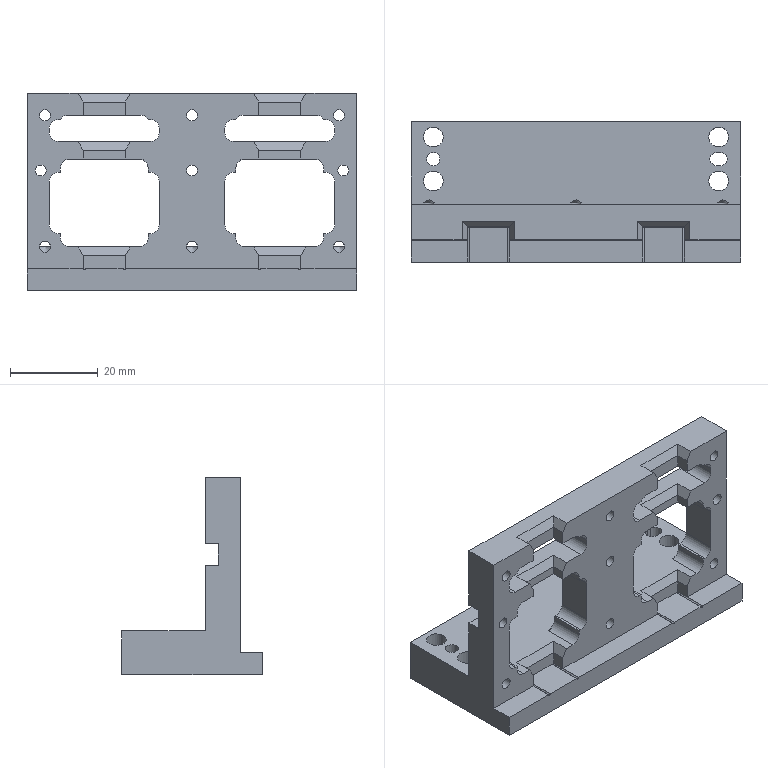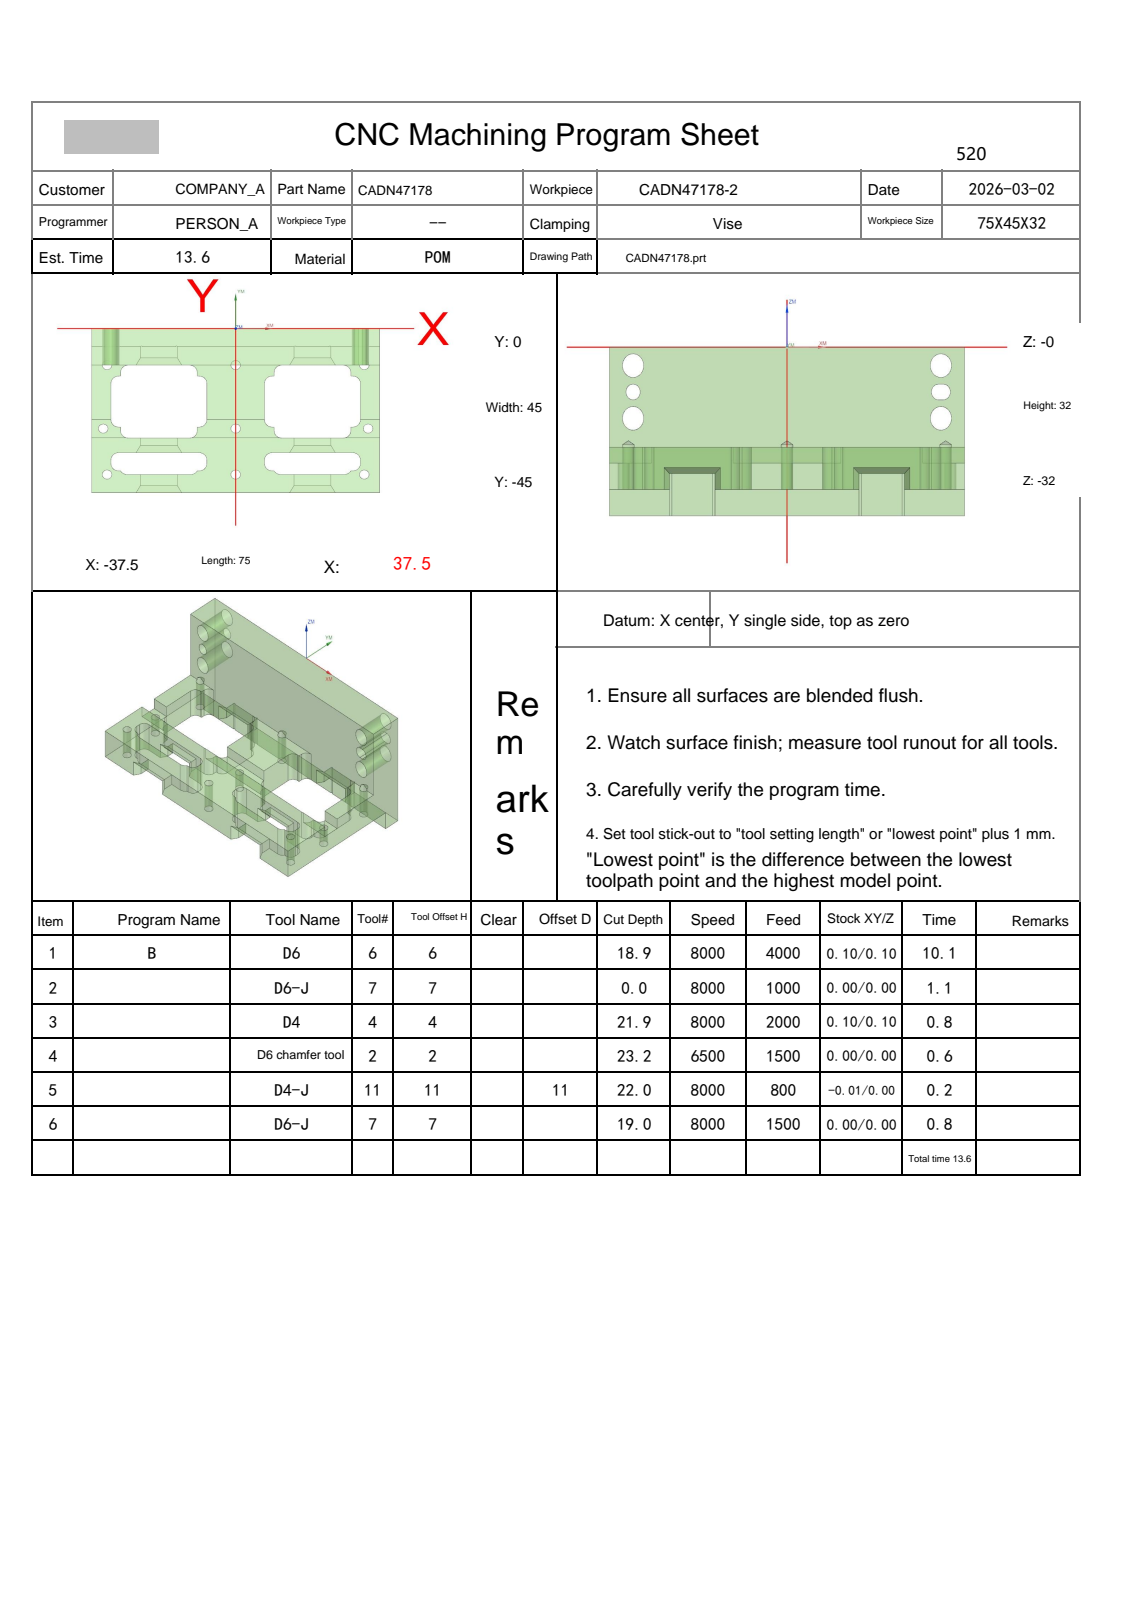NC program | NX | posted by the shop | part box 75 x 32 x 45 mm
Lines 1 to 2828 of 3118, first 1780 of 2826 lines:
%
O0001
(Machine time: 14.54 MIN)
(===Total Tool:5===)
(T6=D6      D=6.   R=0.   D-  H06 Z=-18.9 )
(T7=D6-J    D=6.   R=0.   D-  H07 Z=-19.  )
(T4=D4      D=4.   R=0.   D-  H04 Z=-21.9 )
(T2=D6 chamfer tool   D=6.   R=0.   D-  H02 Z=-23.2 )
(T11=D4-J   D=4.   R=0.   D11 H11 Z=-22.  )
G80 G90 G17 G49 G40
G91 G28 Z0
M01
N1 T06 M06
(D6  D=6. R=0. H=06 ce=0.20 di=0.10)
G00 G90 G54 X52.5 Y-45. M03 S8000
G43 H06 Z50.
M08
Z5.014
G01 Z3.014 F4000.
X40.5
X-39.96
G02 X-40.5 Y-44.46 I0.0 J.54
G01 Y-42.54
G02 X-39.96 Y-42. I.54 J0.0
G01 X39.96
G03 X40.5 Y-41.46 I0.0 J.54
G01 Y-39.54
G03 X39.96 Y-39. I-.54 J0.0
G01 X-39.96
G02 X-40.5 Y-38.46 I0.0 J.54
G01 Y-36.54
G02 X-39.96 Y-36. I.54 J0.0
G01 X39.96
G03 X40.5 Y-35.46 I0.0 J.54
G01 Y-33.54
G03 X39.96 Y-33. I-.54 J0.0
G01 X-39.96
G02 X-40.5 Y-32.46 I0.0 J.54
G01 Y-30.54
G02 X-39.96 Y-30. I.54 J0.0
G01 X39.96
G03 X40.5 Y-29.46 I0.0 J.54
G01 Y-27.54
G03 X39.96 Y-27. I-.54 J0.0
G01 X-39.96
G02 X-40.5 Y-26.46 I0.0 J.54
G01 Y-24.54
G02 X-39.96 Y-24. I.54 J0.0
G01 X39.96
G03 X40.5 Y-23.46 I0.0 J.54
G01 Y-21.54
G03 X39.96 Y-21. I-.54 J0.0
G01 X-39.96
G02 X-40.5 Y-20.46 I0.0 J.54
G01 Y-18.54
G02 X-39.96 Y-18. I.54 J0.0
G01 X39.96
G03 X40.5 Y-17.46 I0.0 J.54
G01 Y-15.54
G03 X39.96 Y-15. I-.54 J0.0
G01 X-39.96
G02 X-40.5 Y-14.46 I0.0 J.54
G01 Y-12.54
G02 X-39.96 Y-12. I.54 J0.0
G01 X39.96
G03 X40.5 Y-11.46 I0.0 J.54
G01 Y-9.54
G03 X39.96 Y-9. I-.54 J0.0
G01 X-39.96
G02 X-40.5 Y-8.46 I0.0 J.54
G01 Y-6.54
G02 X-39.96 Y-6. I.54 J0.0
G01 X39.96
G03 X40.5 Y-5.46 I0.0 J.54
G01 Y-3.54
G03 X39.96 Y-3. I-.54 J0.0
G01 X-39.96
G02 X-40.5 Y-2.46 I0.0 J.54
G01 Y-.54
G02 X-39.96 Y0.0 I.54 J0.0
G01 X40.5
X52.5
Z5.014
G00 Z6.5
Y-45.
Z4.529
G01 Z2.529
X40.5
X-39.96
G02 X-40.5 Y-44.46 I0.0 J.54
G01 Y-42.54
G02 X-39.96 Y-42. I.54 J0.0
G01 X39.96
G03 X40.5 Y-41.46 I0.0 J.54
G01 Y-39.54
G03 X39.96 Y-39. I-.54 J0.0
G01 X-39.96
G02 X-40.5 Y-38.46 I0.0 J.54
G01 Y-36.54
G02 X-39.96 Y-36. I.54 J0.0
G01 X39.96
G03 X40.5 Y-35.46 I0.0 J.54
G01 Y-33.54
G03 X39.96 Y-33. I-.54 J0.0
G01 X-39.96
G02 X-40.5 Y-32.46 I0.0 J.54
G01 Y-30.54
G02 X-39.96 Y-30. I.54 J0.0
G01 X39.96
G03 X40.5 Y-29.46 I0.0 J.54
G01 Y-27.54
G03 X39.96 Y-27. I-.54 J0.0
G01 X-39.96
G02 X-40.5 Y-26.46 I0.0 J.54
G01 Y-24.54
G02 X-39.96 Y-24. I.54 J0.0
G01 X39.96
G03 X40.5 Y-23.46 I0.0 J.54
G01 Y-21.54
G03 X39.96 Y-21. I-.54 J0.0
G01 X-39.96
G02 X-40.5 Y-20.46 I0.0 J.54
G01 Y-18.54
G02 X-39.96 Y-18. I.54 J0.0
G01 X39.96
G03 X40.5 Y-17.46 I0.0 J.54
G01 Y-15.54
G03 X39.96 Y-15. I-.54 J0.0
G01 X-39.96
G02 X-40.5 Y-14.46 I0.0 J.54
G01 Y-12.54
G02 X-39.96 Y-12. I.54 J0.0
G01 X39.96
G03 X40.5 Y-11.46 I0.0 J.54
G01 Y-9.54
G03 X39.96 Y-9. I-.54 J0.0
G01 X-39.96
G02 X-40.5 Y-8.46 I0.0 J.54
G01 Y-6.54
G02 X-39.96 Y-6. I.54 J0.0
G01 X39.96
G03 X40.5 Y-5.46 I0.0 J.54
G01 Y-3.54
G03 X39.96 Y-3. I-.54 J0.0
G01 X-39.96
G02 X-40.5 Y-2.46 I0.0 J.54
G01 Y-.54
G02 X-39.96 Y0.0 I.54 J0.0
G01 X40.5
X52.5
Z4.529
G00 Z6.014
Y-45.
Z4.043
G01 Z2.043
X40.5
X-39.96
G02 X-40.5 Y-44.46 I0.0 J.54
G01 Y-42.54
G02 X-39.96 Y-42. I.54 J0.0
G01 X39.96
G03 X40.5 Y-41.46 I0.0 J.54
G01 Y-39.54
G03 X39.96 Y-39. I-.54 J0.0
G01 X-39.96
G02 X-40.5 Y-38.46 I0.0 J.54
G01 Y-36.54
G02 X-39.96 Y-36. I.54 J0.0
G01 X39.96
G03 X40.5 Y-35.46 I0.0 J.54
G01 Y-33.54
G03 X39.96 Y-33. I-.54 J0.0
G01 X-39.96
G02 X-40.5 Y-32.46 I0.0 J.54
G01 Y-30.54
G02 X-39.96 Y-30. I.54 J0.0
G01 X39.96
G03 X40.5 Y-29.46 I0.0 J.54
G01 Y-27.54
G03 X39.96 Y-27. I-.54 J0.0
G01 X-39.96
G02 X-40.5 Y-26.46 I0.0 J.54
G01 Y-24.54
G02 X-39.96 Y-24. I.54 J0.0
G01 X39.96
G03 X40.5 Y-23.46 I0.0 J.54
G01 Y-21.54
G03 X39.96 Y-21. I-.54 J0.0
G01 X-39.96
G02 X-40.5 Y-20.46 I0.0 J.54
G01 Y-18.54
G02 X-39.96 Y-18. I.54 J0.0
G01 X39.96
G03 X40.5 Y-17.46 I0.0 J.54
G01 Y-15.54
G03 X39.96 Y-15. I-.54 J0.0
G01 X-39.96
G02 X-40.5 Y-14.46 I0.0 J.54
G01 Y-12.54
G02 X-39.96 Y-12. I.54 J0.0
G01 X39.96
G03 X40.5 Y-11.46 I0.0 J.54
G01 Y-9.54
G03 X39.96 Y-9. I-.54 J0.0
G01 X-39.96
G02 X-40.5 Y-8.46 I0.0 J.54
G01 Y-6.54
G02 X-39.96 Y-6. I.54 J0.0
G01 X39.96
G03 X40.5 Y-5.46 I0.0 J.54
G01 Y-3.54
G03 X39.96 Y-3. I-.54 J0.0
G01 X-39.96
G02 X-40.5 Y-2.46 I0.0 J.54
G01 Y-.54
G02 X-39.96 Y0.0 I.54 J0.0
G01 X40.5
X52.5
Z4.043
G00 Z5.529
Y-45.
Z3.557
G01 Z1.557
X40.5
X-39.96
G02 X-40.5 Y-44.46 I0.0 J.54
G01 Y-42.54
G02 X-39.96 Y-42. I.54 J0.0
G01 X39.96
G03 X40.5 Y-41.46 I0.0 J.54
G01 Y-39.54
G03 X39.96 Y-39. I-.54 J0.0
G01 X-39.96
G02 X-40.5 Y-38.46 I0.0 J.54
G01 Y-36.54
G02 X-39.96 Y-36. I.54 J0.0
G01 X39.96
G03 X40.5 Y-35.46 I0.0 J.54
G01 Y-33.54
G03 X39.96 Y-33. I-.54 J0.0
G01 X-39.96
G02 X-40.5 Y-32.46 I0.0 J.54
G01 Y-30.54
G02 X-39.96 Y-30. I.54 J0.0
G01 X39.96
G03 X40.5 Y-29.46 I0.0 J.54
G01 Y-27.54
G03 X39.96 Y-27. I-.54 J0.0
G01 X-39.96
G02 X-40.5 Y-26.46 I0.0 J.54
G01 Y-24.54
G02 X-39.96 Y-24. I.54 J0.0
G01 X39.96
G03 X40.5 Y-23.46 I0.0 J.54
G01 Y-21.54
G03 X39.96 Y-21. I-.54 J0.0
G01 X-39.96
G02 X-40.5 Y-20.46 I0.0 J.54
G01 Y-18.54
G02 X-39.96 Y-18. I.54 J0.0
G01 X39.96
G03 X40.5 Y-17.46 I0.0 J.54
G01 Y-15.54
G03 X39.96 Y-15. I-.54 J0.0
G01 X-39.96
G02 X-40.5 Y-14.46 I0.0 J.54
G01 Y-12.54
G02 X-39.96 Y-12. I.54 J0.0
G01 X39.96
G03 X40.5 Y-11.46 I0.0 J.54
G01 Y-9.54
G03 X39.96 Y-9. I-.54 J0.0
G01 X-39.96
G02 X-40.5 Y-8.46 I0.0 J.54
G01 Y-6.54
G02 X-39.96 Y-6. I.54 J0.0
G01 X39.96
G03 X40.5 Y-5.46 I0.0 J.54
G01 Y-3.54
G03 X39.96 Y-3. I-.54 J0.0
G01 X-39.96
G02 X-40.5 Y-2.46 I0.0 J.54
G01 Y-.54
G02 X-39.96 Y0.0 I.54 J0.0
G01 X40.5
X52.5
Z3.557
G00 Z5.043
Y-45.
Z3.071
G01 Z1.071
X40.5
X-39.96
G02 X-40.5 Y-44.46 I0.0 J.54
G01 Y-42.54
G02 X-39.96 Y-42. I.54 J0.0
G01 X39.96
G03 X40.5 Y-41.46 I0.0 J.54
G01 Y-39.54
G03 X39.96 Y-39. I-.54 J0.0
G01 X-39.96
G02 X-40.5 Y-38.46 I0.0 J.54
G01 Y-36.54
G02 X-39.96 Y-36. I.54 J0.0
G01 X39.96
G03 X40.5 Y-35.46 I0.0 J.54
G01 Y-33.54
G03 X39.96 Y-33. I-.54 J0.0
G01 X-39.96
G02 X-40.5 Y-32.46 I0.0 J.54
G01 Y-30.54
G02 X-39.96 Y-30. I.54 J0.0
G01 X39.96
G03 X40.5 Y-29.46 I0.0 J.54
G01 Y-27.54
G03 X39.96 Y-27. I-.54 J0.0
G01 X-39.96
G02 X-40.5 Y-26.46 I0.0 J.54
G01 Y-24.54
G02 X-39.96 Y-24. I.54 J0.0
G01 X39.96
G03 X40.5 Y-23.46 I0.0 J.54
G01 Y-21.54
G03 X39.96 Y-21. I-.54 J0.0
G01 X-39.96
G02 X-40.5 Y-20.46 I0.0 J.54
G01 Y-18.54
G02 X-39.96 Y-18. I.54 J0.0
G01 X39.96
G03 X40.5 Y-17.46 I0.0 J.54
G01 Y-15.54
G03 X39.96 Y-15. I-.54 J0.0
G01 X-39.96
G02 X-40.5 Y-14.46 I0.0 J.54
G01 Y-12.54
G02 X-39.96 Y-12. I.54 J0.0
G01 X39.96
G03 X40.5 Y-11.46 I0.0 J.54
G01 Y-9.54
G03 X39.96 Y-9. I-.54 J0.0
G01 X-39.96
G02 X-40.5 Y-8.46 I0.0 J.54
G01 Y-6.54
G02 X-39.96 Y-6. I.54 J0.0
G01 X39.96
G03 X40.5 Y-5.46 I0.0 J.54
G01 Y-3.54
G03 X39.96 Y-3. I-.54 J0.0
G01 X-39.96
G02 X-40.5 Y-2.46 I0.0 J.54
G01 Y-.54
G02 X-39.96 Y0.0 I.54 J0.0
G01 X40.5
X52.5
Z3.071
G00 Z4.557
Y-45.
Z2.586
G01 Z.586
X40.5
X-39.96
G02 X-40.5 Y-44.46 I0.0 J.54
G01 Y-42.54
G02 X-39.96 Y-42. I.54 J0.0
G01 X39.96
G03 X40.5 Y-41.46 I0.0 J.54
G01 Y-39.54
G03 X39.96 Y-39. I-.54 J0.0
G01 X-39.96
G02 X-40.5 Y-38.46 I0.0 J.54
G01 Y-36.54
G02 X-39.96 Y-36. I.54 J0.0
G01 X39.96
G03 X40.5 Y-35.46 I0.0 J.54
G01 Y-33.54
G03 X39.96 Y-33. I-.54 J0.0
G01 X-39.96
G02 X-40.5 Y-32.46 I0.0 J.54
G01 Y-30.54
G02 X-39.96 Y-30. I.54 J0.0
G01 X39.96
G03 X40.5 Y-29.46 I0.0 J.54
G01 Y-27.54
G03 X39.96 Y-27. I-.54 J0.0
G01 X-39.96
G02 X-40.5 Y-26.46 I0.0 J.54
G01 Y-24.54
G02 X-39.96 Y-24. I.54 J0.0
G01 X39.96
G03 X40.5 Y-23.46 I0.0 J.54
G01 Y-21.54
G03 X39.96 Y-21. I-.54 J0.0
G01 X-39.96
G02 X-40.5 Y-20.46 I0.0 J.54
G01 Y-18.54
G02 X-39.96 Y-18. I.54 J0.0
G01 X39.96
G03 X40.5 Y-17.46 I0.0 J.54
G01 Y-15.54
G03 X39.96 Y-15. I-.54 J0.0
G01 X-39.96
G02 X-40.5 Y-14.46 I0.0 J.54
G01 Y-12.54
G02 X-39.96 Y-12. I.54 J0.0
G01 X39.96
G03 X40.5 Y-11.46 I0.0 J.54
G01 Y-9.54
G03 X39.96 Y-9. I-.54 J0.0
G01 X-39.96
G02 X-40.5 Y-8.46 I0.0 J.54
G01 Y-6.54
G02 X-39.96 Y-6. I.54 J0.0
G01 X39.96
G03 X40.5 Y-5.46 I0.0 J.54
G01 Y-3.54
G03 X39.96 Y-3. I-.54 J0.0
G01 X-39.96
G02 X-40.5 Y-2.46 I0.0 J.54
G01 Y-.54
G02 X-39.96 Y0.0 I.54 J0.0
G01 X40.5
X52.5
Z2.586
G00 Z4.071
Y-45.
Z2.1
G01 Z.1
X40.5
X-39.96
G02 X-40.5 Y-44.46 I0.0 J.54
G01 Y-42.54
G02 X-39.96 Y-42. I.54 J0.0
G01 X39.96
G03 X40.5 Y-41.46 I0.0 J.54
G01 Y-39.54
G03 X39.96 Y-39. I-.54 J0.0
G01 X-39.96
G02 X-40.5 Y-38.46 I0.0 J.54
G01 Y-36.54
G02 X-39.96 Y-36. I.54 J0.0
G01 X39.96
G03 X40.5 Y-35.46 I0.0 J.54
G01 Y-33.54
G03 X39.96 Y-33. I-.54 J0.0
G01 X-39.96
G02 X-40.5 Y-32.46 I0.0 J.54
G01 Y-30.54
G02 X-39.96 Y-30. I.54 J0.0
G01 X39.96
G03 X40.5 Y-29.46 I0.0 J.54
G01 Y-27.54
G03 X39.96 Y-27. I-.54 J0.0
G01 X-39.96
G02 X-40.5 Y-26.46 I0.0 J.54
G01 Y-24.54
G02 X-39.96 Y-24. I.54 J0.0
G01 X39.96
G03 X40.5 Y-23.46 I0.0 J.54
G01 Y-21.54
G03 X39.96 Y-21. I-.54 J0.0
G01 X-39.96
G02 X-40.5 Y-20.46 I0.0 J.54
G01 Y-18.54
G02 X-39.96 Y-18. I.54 J0.0
G01 X39.96
G03 X40.5 Y-17.46 I0.0 J.54
G01 Y-15.54
G03 X39.96 Y-15. I-.54 J0.0
G01 X-39.96
G02 X-40.5 Y-14.46 I0.0 J.54
G01 Y-12.54
G02 X-39.96 Y-12. I.54 J0.0
G01 X39.96
G03 X40.5 Y-11.46 I0.0 J.54
G01 Y-9.54
G03 X39.96 Y-9. I-.54 J0.0
G01 X-39.96
G02 X-40.5 Y-8.46 I0.0 J.54
G01 Y-6.54
G02 X-39.96 Y-6. I.54 J0.0
G01 X39.96
G03 X40.5 Y-5.46 I0.0 J.54
G01 Y-3.54
G03 X39.96 Y-3. I-.54 J0.0
G01 X-39.96
G02 X-40.5 Y-2.46 I0.0 J.54
G01 Y-.54
G02 X-39.96 Y0.0 I.54 J0.0
G01 X40.5
X52.5
Z2.1
G00 Z50.
G00 G90 X43.5 Y-47.6 M03 S8000
Z12.5
Z1.003
G01 Z-.497 F4000.
X40.44
X-39.9
G02 X-40.44 Y-47.06 I0.0 J.54
G01 Y-45.2
G02 X-39.84 Y-44.6 I.6 J0.0
G01 X39.84
G03 X40.44 Y-44. I0.0 J.6
G01 Y-40.7
G03 X39.84 Y-40.1 I-.6 J0.0
G01 X-39.84
G02 X-40.44 Y-39.5 I0.0 J.6
G01 Y-36.199
G02 X-39.84 Y-35.6 I.6 J-.001
G01 X39.841
G03 X40.44 Y-35.001 I-.001 J.6
G01 Y-31.699
G03 X39.841 Y-31.1 I-.6 J-.001
G01 X-39.84
G02 X-40.44 Y-30.5 I0.0 J.6
G01 Y-27.199
G02 X-39.84 Y-26.6 I.6 J-.001
G01 X39.841
G03 X40.44 Y-26.001 I-.001 J.6
G01 Y-22.699
G03 X39.84 Y-22.1 I-.6 J-.001
G01 X-39.841
G02 X-40.44 Y-21.5 I.001 J.6
G01 Y-18.2
G02 X-39.84 Y-17.6 I.6 J0.0
G01 X39.927
G03 X40.519 Y-17.093 I-.001 J.6
G01 X41.033 Y-13.792
X41.04 Y-13.7
G03 X40.44 Y-13.1 I-.6 J0.0
G01 X-40.44
X-43.6
Z1.003
G00 X43.5 Y-47.6
Z.505
G01 Z-.995
X40.44
X-39.9
G02 X-40.44 Y-47.06 I0.0 J.54
G01 Y-45.2
G02 X-39.84 Y-44.6 I.6 J0.0
G01 X39.84
G03 X40.44 Y-44. I0.0 J.6
G01 Y-40.7
G03 X39.84 Y-40.1 I-.6 J0.0
G01 X-39.84
G02 X-40.44 Y-39.5 I0.0 J.6
G01 Y-36.199
G02 X-39.84 Y-35.6 I.6 J-.001
G01 X39.841
G03 X40.44 Y-35.001 I-.001 J.6
G01 Y-31.699
G03 X39.841 Y-31.1 I-.6 J-.001
G01 X-39.84
G02 X-40.44 Y-30.5 I0.0 J.6
G01 Y-27.199
G02 X-39.84 Y-26.6 I.6 J-.001
G01 X39.841
G03 X40.44 Y-26.001 I-.001 J.6
G01 Y-22.699
G03 X39.84 Y-22.1 I-.6 J-.001
G01 X-39.841
G02 X-40.44 Y-21.5 I.001 J.6
G01 Y-18.2
G02 X-39.84 Y-17.6 I.6 J0.0
G01 X39.927
G03 X40.519 Y-17.093 I-.001 J.6
G01 X41.033 Y-13.792
X41.04 Y-13.7
G03 X40.44 Y-13.1 I-.6 J0.0
G01 X-40.44
X-43.6
Z.505
G00 X43.5 Y-47.6
Z.008
G01 Z-1.492
X40.44
X-39.9
G02 X-40.44 Y-47.06 I0.0 J.54
G01 Y-45.2
G02 X-39.84 Y-44.6 I.6 J0.0
G01 X39.84
G03 X40.44 Y-44. I0.0 J.6
G01 Y-40.7
G03 X39.84 Y-40.1 I-.6 J0.0
G01 X-39.84
G02 X-40.44 Y-39.5 I0.0 J.6
G01 Y-36.199
G02 X-39.84 Y-35.6 I.6 J-.001
G01 X39.841
G03 X40.44 Y-35.001 I-.001 J.6
G01 Y-31.699
G03 X39.841 Y-31.1 I-.6 J-.001
G01 X-39.84
G02 X-40.44 Y-30.5 I0.0 J.6
G01 Y-27.199
G02 X-39.84 Y-26.6 I.6 J-.001
G01 X39.841
G03 X40.44 Y-26.001 I-.001 J.6
G01 Y-22.699
G03 X39.84 Y-22.1 I-.6 J-.001
G01 X-39.841
G02 X-40.44 Y-21.5 I.001 J.6
G01 Y-18.2
G02 X-39.84 Y-17.6 I.6 J0.0
G01 X39.927
G03 X40.519 Y-17.093 I-.001 J.6
G01 X41.033 Y-13.792
X41.04 Y-13.7
G03 X40.44 Y-13.1 I-.6 J0.0
G01 X-40.44
X-43.6
Z.008
G00 X43.5 Y-47.6
Z-.489
G01 Z-1.989
X40.44
X-39.9
G02 X-40.44 Y-47.06 I0.0 J.54
G01 Y-45.2
G02 X-39.84 Y-44.6 I.6 J0.0
G01 X39.84
G03 X40.44 Y-44. I0.0 J.6
G01 Y-40.7
G03 X39.84 Y-40.1 I-.6 J0.0
G01 X-39.84
G02 X-40.44 Y-39.5 I0.0 J.6
G01 Y-36.199
G02 X-39.84 Y-35.6 I.6 J-.001
G01 X39.841
G03 X40.44 Y-35.001 I-.001 J.6
G01 Y-31.699
G03 X39.841 Y-31.1 I-.6 J-.001
G01 X-39.84
G02 X-40.44 Y-30.5 I0.0 J.6
G01 Y-27.199
G02 X-39.84 Y-26.6 I.6 J-.001
G01 X39.841
G03 X40.44 Y-26.001 I-.001 J.6
G01 Y-22.699
G03 X39.84 Y-22.1 I-.6 J-.001
G01 X-39.841
G02 X-40.44 Y-21.5 I.001 J.6
G01 Y-18.2
G02 X-39.84 Y-17.6 I.6 J0.0
G01 X39.927
G03 X40.519 Y-17.093 I-.001 J.6
G01 X41.033 Y-13.792
X41.04 Y-13.7
G03 X40.44 Y-13.1 I-.6 J0.0
G01 X-40.44
X-43.6
Z-.489
G00 X43.5 Y-47.6
Z-.987
G01 Z-2.487
X40.44
X-39.9
G02 X-40.44 Y-47.06 I0.0 J.54
G01 Y-45.2
G02 X-39.84 Y-44.6 I.6 J0.0
G01 X39.84
G03 X40.44 Y-44. I0.0 J.6
G01 Y-40.7
G03 X39.84 Y-40.1 I-.6 J0.0
G01 X-39.84
G02 X-40.44 Y-39.5 I0.0 J.6
G01 Y-36.199
G02 X-39.84 Y-35.6 I.6 J-.001
G01 X39.841
G03 X40.44 Y-35.001 I-.001 J.6
G01 Y-31.699
G03 X39.841 Y-31.1 I-.6 J-.001
G01 X-39.84
G02 X-40.44 Y-30.5 I0.0 J.6
G01 Y-27.199
G02 X-39.84 Y-26.6 I.6 J-.001
G01 X39.841
G03 X40.44 Y-26.001 I-.001 J.6
G01 Y-22.699
G03 X39.84 Y-22.1 I-.6 J-.001
G01 X-39.841
G02 X-40.44 Y-21.5 I.001 J.6
G01 Y-18.2
G02 X-39.84 Y-17.6 I.6 J0.0
G01 X39.927
G03 X40.519 Y-17.093 I-.001 J.6
G01 X41.033 Y-13.792
X41.04 Y-13.7
G03 X40.44 Y-13.1 I-.6 J0.0
G01 X-40.44
X-43.6
Z-.987
G00 X43.5 Y-47.6
Z-1.484
G01 Z-2.984
X40.44
X-39.9
G02 X-40.44 Y-47.06 I0.0 J.54
G01 Y-45.2
G02 X-39.84 Y-44.6 I.6 J0.0
G01 X39.84
G03 X40.44 Y-44. I0.0 J.6
G01 Y-40.7
G03 X39.84 Y-40.1 I-.6 J0.0
G01 X-39.84
G02 X-40.44 Y-39.5 I0.0 J.6
G01 Y-36.199
G02 X-39.84 Y-35.6 I.6 J-.001
G01 X39.841
G03 X40.44 Y-35.001 I-.001 J.6
G01 Y-31.699
G03 X39.841 Y-31.1 I-.6 J-.001
G01 X-39.84
G02 X-40.44 Y-30.5 I0.0 J.6
G01 Y-27.199
G02 X-39.84 Y-26.6 I.6 J-.001
G01 X39.841
G03 X40.44 Y-26.001 I-.001 J.6
G01 Y-22.699
G03 X39.84 Y-22.1 I-.6 J-.001
G01 X-39.841
G02 X-40.44 Y-21.5 I.001 J.6
G01 Y-18.2
G02 X-39.84 Y-17.6 I.6 J0.0
G01 X39.927
G03 X40.519 Y-17.093 I-.001 J.6
G01 X41.033 Y-13.792
X41.04 Y-13.7
G03 X40.44 Y-13.1 I-.6 J0.0
G01 X-40.44
X-43.6
Z-1.484
G00 X43.5 Y-47.6
Z-1.982
G01 Z-3.482
X40.44
X-39.9
G02 X-40.44 Y-47.06 I0.0 J.54
G01 Y-45.2
G02 X-39.84 Y-44.6 I.6 J0.0
G01 X39.84
G03 X40.44 Y-44. I0.0 J.6
G01 Y-40.7
G03 X39.84 Y-40.1 I-.6 J0.0
G01 X-39.84
G02 X-40.44 Y-39.5 I0.0 J.6
G01 Y-36.199
G02 X-39.84 Y-35.6 I.6 J-.001
G01 X39.841
G03 X40.44 Y-35.001 I-.001 J.6
G01 Y-31.699
G03 X39.841 Y-31.1 I-.6 J-.001
G01 X-39.84
G02 X-40.44 Y-30.5 I0.0 J.6
G01 Y-27.199
G02 X-39.84 Y-26.6 I.6 J-.001
G01 X39.841
G03 X40.44 Y-26.001 I-.001 J.6
G01 Y-22.699
G03 X39.84 Y-22.1 I-.6 J-.001
G01 X-39.841
G02 X-40.44 Y-21.5 I.001 J.6
G01 Y-18.2
G02 X-39.84 Y-17.6 I.6 J0.0
G01 X39.927
G03 X40.519 Y-17.093 I-.001 J.6
G01 X41.033 Y-13.792
X41.04 Y-13.7
G03 X40.44 Y-13.1 I-.6 J0.0
G01 X-40.44
X-43.6
Z-1.982
G00 X43.5 Y-47.6
Z-2.479
G01 Z-3.979
X40.44
X-39.9
G02 X-40.44 Y-47.06 I0.0 J.54
G01 Y-45.2
G02 X-39.84 Y-44.6 I.6 J0.0
G01 X39.84
G03 X40.44 Y-44. I0.0 J.6
G01 Y-40.7
G03 X39.84 Y-40.1 I-.6 J0.0
G01 X-39.84
G02 X-40.44 Y-39.5 I0.0 J.6
G01 Y-36.199
G02 X-39.84 Y-35.6 I.6 J-.001
G01 X39.841
G03 X40.44 Y-35.001 I-.001 J.6
G01 Y-31.699
G03 X39.841 Y-31.1 I-.6 J-.001
G01 X-39.84
G02 X-40.44 Y-30.5 I0.0 J.6
G01 Y-27.199
G02 X-39.84 Y-26.6 I.6 J-.001
G01 X39.841
G03 X40.44 Y-26.001 I-.001 J.6
G01 Y-22.699
G03 X39.84 Y-22.1 I-.6 J-.001
G01 X-39.841
G02 X-40.44 Y-21.5 I.001 J.6
G01 Y-18.2
G02 X-39.84 Y-17.6 I.6 J0.0
G01 X39.927
G03 X40.519 Y-17.093 I-.001 J.6
G01 X41.033 Y-13.792
X41.04 Y-13.7
G03 X40.44 Y-13.1 I-.6 J0.0
G01 X-40.44
X-43.6
Z-2.479
G00 X43.5 Y-47.6
Z-2.976
G01 Z-4.476
X40.44
X-39.9
G02 X-40.44 Y-47.06 I0.0 J.54
G01 Y-45.2
G02 X-39.84 Y-44.6 I.6 J0.0
G01 X39.84
G03 X40.44 Y-44. I0.0 J.6
G01 Y-40.7
G03 X39.84 Y-40.1 I-.6 J0.0
G01 X-39.84
G02 X-40.44 Y-39.5 I0.0 J.6
G01 Y-36.199
G02 X-39.84 Y-35.6 I.6 J-.001
G01 X39.841
G03 X40.44 Y-35.001 I-.001 J.6
G01 Y-31.699
G03 X39.841 Y-31.1 I-.6 J-.001
G01 X-39.84
G02 X-40.44 Y-30.5 I0.0 J.6
G01 Y-27.199
G02 X-39.84 Y-26.6 I.6 J-.001
G01 X39.841
G03 X40.44 Y-26.001 I-.001 J.6
G01 Y-22.699
G03 X39.84 Y-22.1 I-.6 J-.001
G01 X-39.841
G02 X-40.44 Y-21.5 I.001 J.6
G01 Y-18.2
G02 X-39.84 Y-17.6 I.6 J0.0
G01 X39.927
G03 X40.519 Y-17.093 I-.001 J.6
G01 X41.033 Y-13.792
X41.04 Y-13.7
G03 X40.44 Y-13.1 I-.6 J0.0
G01 X-40.44
X-43.6
Z-2.976
G00 X43.5 Y-47.6
Z-3.474
G01 Z-4.974
X40.44
X-39.9
G02 X-40.44 Y-47.06 I0.0 J.54
G01 Y-45.2
G02 X-39.84 Y-44.6 I.6 J0.0
G01 X39.84
G03 X40.44 Y-44. I0.0 J.6
G01 Y-40.7
G03 X39.84 Y-40.1 I-.6 J0.0
G01 X-39.84
G02 X-40.44 Y-39.5 I0.0 J.6
G01 Y-36.199
G02 X-39.84 Y-35.6 I.6 J-.001
G01 X39.841
G03 X40.44 Y-35.001 I-.001 J.6
G01 Y-31.699
G03 X39.841 Y-31.1 I-.6 J-.001
G01 X-39.84
G02 X-40.44 Y-30.5 I0.0 J.6
G01 Y-27.199
G02 X-39.84 Y-26.6 I.6 J-.001
G01 X39.841
G03 X40.44 Y-26.001 I-.001 J.6
G01 Y-22.699
G03 X39.84 Y-22.1 I-.6 J-.001
G01 X-39.841
G02 X-40.44 Y-21.5 I.001 J.6
G01 Y-18.2
G02 X-39.84 Y-17.6 I.6 J0.0
G01 X39.927
G03 X40.519 Y-17.093 I-.001 J.6
G01 X41.033 Y-13.792
X41.04 Y-13.7
G03 X40.44 Y-13.1 I-.6 J0.0
G01 X-40.44
X-43.6
Z-3.474
G00 X43.5 Y-47.6
Z-3.971
G01 Z-5.471
X40.44
X-39.9
G02 X-40.44 Y-47.06 I0.0 J.54
G01 Y-45.2
G02 X-39.84 Y-44.6 I.6 J0.0
G01 X39.84
G03 X40.44 Y-44. I0.0 J.6
G01 Y-40.7
G03 X39.84 Y-40.1 I-.6 J0.0
G01 X-39.84
G02 X-40.44 Y-39.5 I0.0 J.6
G01 Y-36.199
G02 X-39.84 Y-35.6 I.6 J-.001
G01 X39.841
G03 X40.44 Y-35.001 I-.001 J.6
G01 Y-31.699
G03 X39.841 Y-31.1 I-.6 J-.001
G01 X-39.84
G02 X-40.44 Y-30.5 I0.0 J.6
G01 Y-27.199
G02 X-39.84 Y-26.6 I.6 J-.001
G01 X39.841
G03 X40.44 Y-26.001 I-.001 J.6
G01 Y-22.699
G03 X39.84 Y-22.1 I-.6 J-.001
G01 X-39.841
G02 X-40.44 Y-21.5 I.001 J.6
G01 Y-18.2
G02 X-39.84 Y-17.6 I.6 J0.0
G01 X39.927
G03 X40.519 Y-17.093 I-.001 J.6
G01 X41.033 Y-13.792
X41.04 Y-13.7
G03 X40.44 Y-13.1 I-.6 J0.0
G01 X-40.44
X-43.6
Z-3.971
G00 X43.5 Y-47.6
Z-4.468
G01 Z-5.968
X40.44
X-39.9
G02 X-40.44 Y-47.06 I0.0 J.54
G01 Y-45.2
G02 X-39.84 Y-44.6 I.6 J0.0
G01 X39.84
G03 X40.44 Y-44. I0.0 J.6
G01 Y-40.7
G03 X39.84 Y-40.1 I-.6 J0.0
G01 X-39.84
G02 X-40.44 Y-39.5 I0.0 J.6
G01 Y-36.199
G02 X-39.84 Y-35.6 I.6 J-.001
G01 X39.841
G03 X40.44 Y-35.001 I-.001 J.6
G01 Y-31.699
G03 X39.841 Y-31.1 I-.6 J-.001
G01 X-39.84
G02 X-40.44 Y-30.5 I0.0 J.6
G01 Y-27.199
G02 X-39.84 Y-26.6 I.6 J-.001
G01 X39.841
G03 X40.44 Y-26.001 I-.001 J.6
G01 Y-22.699
G03 X39.84 Y-22.1 I-.6 J-.001
G01 X-39.841
G02 X-40.44 Y-21.5 I.001 J.6
G01 Y-18.2
G02 X-39.84 Y-17.6 I.6 J0.0
G01 X39.927
G03 X40.519 Y-17.093 I-.001 J.6
G01 X41.033 Y-13.792
X41.04 Y-13.7
G03 X40.44 Y-13.1 I-.6 J0.0
G01 X-40.44
X-43.6
Z-4.468
G00 X43.5 Y-47.6
Z-4.966
G01 Z-6.466
X40.44
X-39.9
G02 X-40.44 Y-47.06 I0.0 J.54
G01 Y-45.2
G02 X-39.84 Y-44.6 I.6 J0.0
G01 X39.84
G03 X40.44 Y-44. I0.0 J.6
G01 Y-40.7
G03 X39.84 Y-40.1 I-.6 J0.0
G01 X-39.84
G02 X-40.44 Y-39.5 I0.0 J.6
G01 Y-36.199
G02 X-39.84 Y-35.6 I.6 J-.001
G01 X39.841
G03 X40.44 Y-35.001 I-.001 J.6
G01 Y-31.699
G03 X39.841 Y-31.1 I-.6 J-.001
G01 X-39.84
G02 X-40.44 Y-30.5 I0.0 J.6
G01 Y-27.199
G02 X-39.84 Y-26.6 I.6 J-.001
G01 X39.841
G03 X40.44 Y-26.001 I-.001 J.6
G01 Y-22.699
G03 X39.84 Y-22.1 I-.6 J-.001
G01 X-39.841
G02 X-40.44 Y-21.5 I.001 J.6
G01 Y-18.2
G02 X-39.84 Y-17.6 I.6 J0.0
G01 X39.927
G03 X40.519 Y-17.093 I-.001 J.6
G01 X41.033 Y-13.792
X41.04 Y-13.7
G03 X40.44 Y-13.1 I-.6 J0.0
G01 X-40.44
X-43.6
Z-4.966
G00 X43.5 Y-47.6
Z-5.463
G01 Z-6.963
X40.44
X-39.9
G02 X-40.44 Y-47.06 I0.0 J.54
G01 Y-45.2
G02 X-39.84 Y-44.6 I.6 J0.0
G01 X39.84
G03 X40.44 Y-44. I0.0 J.6
G01 Y-40.7
G03 X39.84 Y-40.1 I-.6 J0.0
G01 X-39.84
G02 X-40.44 Y-39.5 I0.0 J.6
G01 Y-36.199
G02 X-39.84 Y-35.6 I.6 J-.001
G01 X39.841
G03 X40.44 Y-35.001 I-.001 J.6
G01 Y-31.699
G03 X39.841 Y-31.1 I-.6 J-.001
G01 X-39.84
G02 X-40.44 Y-30.5 I0.0 J.6
G01 Y-27.199
G02 X-39.84 Y-26.6 I.6 J-.001
G01 X39.841
G03 X40.44 Y-26.001 I-.001 J.6
G01 Y-22.699
G03 X39.84 Y-22.1 I-.6 J-.001
G01 X-39.841
G02 X-40.44 Y-21.5 I.001 J.6
G01 Y-18.2
G02 X-39.84 Y-17.6 I.6 J0.0
G01 X39.927
G03 X40.519 Y-17.093 I-.001 J.6
G01 X41.033 Y-13.792
X41.04 Y-13.7
G03 X40.44 Y-13.1 I-.6 J0.0
G01 X-40.44
X-43.6
Z-5.463
G00 X43.5 Y-47.6
Z-5.961
G01 Z-7.461
X40.44
X-39.9
G02 X-40.44 Y-47.06 I0.0 J.54
G01 Y-45.2
G02 X-39.84 Y-44.6 I.6 J0.0
G01 X39.84
G03 X40.44 Y-44. I0.0 J.6
G01 Y-40.7
G03 X39.84 Y-40.1 I-.6 J0.0
G01 X-39.84
G02 X-40.44 Y-39.5 I0.0 J.6
G01 Y-36.199
G02 X-39.84 Y-35.6 I.6 J-.001
G01 X39.841
G03 X40.44 Y-35.001 I-.001 J.6
G01 Y-31.699
G03 X39.841 Y-31.1 I-.6 J-.001
G01 X-39.84
G02 X-40.44 Y-30.5 I0.0 J.6
G01 Y-27.199
G02 X-39.84 Y-26.6 I.6 J-.001
G01 X39.841
G03 X40.44 Y-26.001 I-.001 J.6
G01 Y-22.699
G03 X39.84 Y-22.1 I-.6 J-.001
G01 X-39.841
G02 X-40.44 Y-21.5 I.001 J.6
G01 Y-18.2
G02 X-39.84 Y-17.6 I.6 J0.0
G01 X39.927
G03 X40.519 Y-17.093 I-.001 J.6
G01 X41.033 Y-13.792
X41.04 Y-13.7
G03 X40.44 Y-13.1 I-.6 J0.0
G01 X-40.44
X-43.6
Z-5.961
G00 X43.5 Y-47.6
Z-6.458
G01 Z-7.958
X40.44
X-39.9
G02 X-40.44 Y-47.06 I0.0 J.54
G01 Y-45.2
G02 X-39.84 Y-44.6 I.6 J0.0
G01 X39.84
G03 X40.44 Y-44. I0.0 J.6
G01 Y-40.7
G03 X39.84 Y-40.1 I-.6 J0.0
G01 X-39.84
G02 X-40.44 Y-39.5 I0.0 J.6
G01 Y-36.199
G02 X-39.84 Y-35.6 I.6 J-.001
G01 X39.841
G03 X40.44 Y-35.001 I-.001 J.6
G01 Y-31.699
G03 X39.841 Y-31.1 I-.6 J-.001
G01 X-39.84
G02 X-40.44 Y-30.5 I0.0 J.6
G01 Y-27.199
G02 X-39.84 Y-26.6 I.6 J-.001
G01 X39.841
G03 X40.44 Y-26.001 I-.001 J.6
G01 Y-22.699
G03 X39.84 Y-22.1 I-.6 J-.001
G01 X-39.841
G02 X-40.44 Y-21.5 I.001 J.6
G01 Y-18.2
G02 X-39.84 Y-17.6 I.6 J0.0
G01 X39.927
G03 X40.519 Y-17.093 I-.001 J.6
G01 X41.033 Y-13.792
X41.04 Y-13.7
G03 X40.44 Y-13.1 I-.6 J0.0
G01 X-40.44
X-43.6
Z-6.458
G00 X43.5 Y-47.6
Z-6.955
G01 Z-8.455
X40.44
X-39.9
G02 X-40.44 Y-47.06 I0.0 J.54
G01 Y-45.2
G02 X-39.84 Y-44.6 I.6 J0.0
G01 X39.84
G03 X40.44 Y-44. I0.0 J.6
G01 Y-40.7
G03 X39.84 Y-40.1 I-.6 J0.0
G01 X-39.84
G02 X-40.44 Y-39.5 I0.0 J.6
G01 Y-36.199
G02 X-39.84 Y-35.6 I.6 J-.001
G01 X39.841
G03 X40.44 Y-35.001 I-.001 J.6
G01 Y-31.699
G03 X39.841 Y-31.1 I-.6 J-.001
G01 X-39.84
G02 X-40.44 Y-30.5 I0.0 J.6
G01 Y-27.199
G02 X-39.84 Y-26.6 I.6 J-.001
G01 X39.841
G03 X40.44 Y-26.001 I-.001 J.6
G01 Y-22.699
G03 X39.84 Y-22.1 I-.6 J-.001
G01 X-39.841
G02 X-40.44 Y-21.5 I.001 J.6
G01 Y-18.2
G02 X-39.84 Y-17.6 I.6 J0.0
G01 X39.927
G03 X40.519 Y-17.093 I-.001 J.6
G01 X41.033 Y-13.792
X41.04 Y-13.7
G03 X40.44 Y-13.1 I-.6 J0.0
G01 X-40.44
X-43.6
Z-6.955
G00 X43.5 Y-47.6
Z-7.453
G01 Z-8.953
X40.44
X-39.9
G02 X-40.44 Y-47.06 I0.0 J.54
G01 Y-45.2
G02 X-39.84 Y-44.6 I.6 J0.0
G01 X39.84
G03 X40.44 Y-44. I0.0 J.6
G01 Y-40.7
G03 X39.84 Y-40.1 I-.6 J0.0
G01 X-39.84
G02 X-40.44 Y-39.5 I0.0 J.6
G01 Y-36.199
G02 X-39.84 Y-35.6 I.6 J-.001
G01 X39.841
G03 X40.44 Y-35.001 I-.001 J.6
G01 Y-31.699
G03 X39.841 Y-31.1 I-.6 J-.001
G01 X-39.84
G02 X-40.44 Y-30.5 I0.0 J.6
G01 Y-27.199
G02 X-39.84 Y-26.6 I.6 J-.001
G01 X39.841
G03 X40.44 Y-26.001 I-.001 J.6
G01 Y-22.699
G03 X39.84 Y-22.1 I-.6 J-.001
G01 X-39.841
G02 X-40.44 Y-21.5 I.001 J.6
G01 Y-18.2
G02 X-39.84 Y-17.6 I.6 J0.0
G01 X39.927
G03 X40.519 Y-17.093 I-.001 J.6
G01 X41.033 Y-13.792
X41.04 Y-13.7
G03 X40.44 Y-13.1 I-.6 J0.0
G01 X-40.44
X-43.6
Z-7.453
G00 X43.5 Y-47.6
Z-7.95
G01 Z-9.45
X40.44
X-39.9
G02 X-40.44 Y-47.06 I0.0 J.54
G01 Y-45.2
G02 X-39.84 Y-44.6 I.6 J0.0
G01 X39.84
G03 X40.44 Y-44. I0.0 J.6
G01 Y-40.7
G03 X39.84 Y-40.1 I-.6 J0.0
G01 X-39.84
G02 X-40.44 Y-39.5 I0.0 J.6
G01 Y-36.199
G02 X-39.84 Y-35.6 I.6 J-.001
G01 X39.841
G03 X40.44 Y-35.001 I-.001 J.6
G01 Y-31.699
G03 X39.841 Y-31.1 I-.6 J-.001
G01 X-39.84
G02 X-40.44 Y-30.5 I0.0 J.6
G01 Y-27.199
G02 X-39.84 Y-26.6 I.6 J-.001
G01 X39.841
G03 X40.44 Y-26.001 I-.001 J.6
G01 Y-22.699
G03 X39.84 Y-22.1 I-.6 J-.001
G01 X-39.841
G02 X-40.44 Y-21.5 I.001 J.6
G01 Y-18.2
G02 X-39.84 Y-17.6 I.6 J0.0
G01 X39.927
G03 X40.519 Y-17.093 I-.001 J.6
G01 X41.033 Y-13.792
X41.04 Y-13.7
G03 X40.44 Y-13.1 I-.6 J0.0
G01 X-40.44
X-43.6
Z-7.95
G00 X43.5 Y-47.6
Z-8.447
G01 Z-9.947
X40.44
X-39.9
G02 X-40.44 Y-47.06 I0.0 J.54
G01 Y-45.2
G02 X-39.84 Y-44.6 I.6 J0.0
G01 X39.84
G03 X40.44 Y-44. I0.0 J.6
G01 Y-40.7
G03 X39.84 Y-40.1 I-.6 J0.0
G01 X-39.84
G02 X-40.44 Y-39.5 I0.0 J.6
G01 Y-36.199
G02 X-39.84 Y-35.6 I.6 J-.001
G01 X39.841
G03 X40.44 Y-35.001 I-.001 J.6
G01 Y-31.699
G03 X39.841 Y-31.1 I-.6 J-.001
G01 X-39.84
G02 X-40.44 Y-30.5 I0.0 J.6
G01 Y-27.199
G02 X-39.84 Y-26.6 I.6 J-.001
G01 X39.841
G03 X40.44 Y-26.001 I-.001 J.6
G01 Y-22.699
G03 X39.84 Y-22.1 I-.6 J-.001
G01 X-39.841
G02 X-40.44 Y-21.5 I.001 J.6
G01 Y-18.2
G02 X-39.84 Y-17.6 I.6 J0.0
G01 X39.927
G03 X40.519 Y-17.093 I-.001 J.6
G01 X41.033 Y-13.792
X41.04 Y-13.7
G03 X40.44 Y-13.1 I-.6 J0.0
G01 X-40.44
X-43.6
Z-8.447
G00 X43.5 Y-47.6
Z-8.945
G01 Z-10.445
X40.44
X-39.9
G02 X-40.44 Y-47.06 I0.0 J.54
G01 Y-45.2
G02 X-39.84 Y-44.6 I.6 J0.0
G01 X39.84
G03 X40.44 Y-44. I0.0 J.6
G01 Y-40.7
G03 X39.84 Y-40.1 I-.6 J0.0
G01 X-39.84
G02 X-40.44 Y-39.5 I0.0 J.6
G01 Y-36.199
G02 X-39.84 Y-35.6 I.6 J-.001
G01 X39.841
G03 X40.44 Y-35.001 I-.001 J.6
G01 Y-31.699
G03 X39.841 Y-31.1 I-.6 J-.001
G01 X-39.84
G02 X-40.44 Y-30.5 I0.0 J.6
G01 Y-27.199
G02 X-39.84 Y-26.6 I.6 J-.001
G01 X39.841
G03 X40.44 Y-26.001 I-.001 J.6
G01 Y-22.699
G03 X39.84 Y-22.1 I-.6 J-.001
G01 X-39.841
G02 X-40.44 Y-21.5 I.001 J.6
G01 Y-18.2
G02 X-39.84 Y-17.6 I.6 J0.0
G01 X39.927
G03 X40.519 Y-17.093 I-.001 J.6
G01 X41.033 Y-13.792
X41.04 Y-13.7
G03 X40.44 Y-13.1 I-.6 J0.0
G01 X-40.44
X-43.6
Z-8.945
G00 X43.5 Y-47.6
Z-9.442
G01 Z-10.942
X40.44
X-39.9
G02 X-40.44 Y-47.06 I0.0 J.54
G01 Y-45.2
G02 X-39.84 Y-44.6 I.6 J0.0
G01 X39.84
G03 X40.44 Y-44. I0.0 J.6
G01 Y-40.7
G03 X39.84 Y-40.1 I-.6 J0.0
G01 X-39.84
G02 X-40.44 Y-39.5 I0.0 J.6
G01 Y-36.199
G02 X-39.84 Y-35.6 I.6 J-.001
G01 X39.841
G03 X40.44 Y-35.001 I-.001 J.6
G01 Y-31.699
G03 X39.841 Y-31.1 I-.6 J-.001
G01 X-39.84
G02 X-40.44 Y-30.5 I0.0 J.6
G01 Y-27.199
G02 X-39.84 Y-26.6 I.6 J-.001
G01 X39.841
G03 X40.44 Y-26.001 I-.001 J.6
G01 Y-22.699
G03 X39.84 Y-22.1 I-.6 J-.001
G01 X-39.841
G02 X-40.44 Y-21.5 I.001 J.6
G01 Y-18.2
G02 X-39.84 Y-17.6 I.6 J0.0
G01 X39.927
G03 X40.519 Y-17.093 I-.001 J.6
G01 X41.033 Y-13.792
X41.04 Y-13.7
G03 X40.44 Y-13.1 I-.6 J0.0
G01 X-40.44
X-43.6
Z-9.442
G00 X43.5 Y-47.6
Z-9.939
G01 Z-11.439
X40.44
X-39.9
G02 X-40.44 Y-47.06 I0.0 J.54
G01 Y-45.2
G02 X-39.84 Y-44.6 I.6 J0.0
G01 X39.84
G03 X40.44 Y-44. I0.0 J.6
G01 Y-40.7
G03 X39.84 Y-40.1 I-.6 J0.0
G01 X-39.84
G02 X-40.44 Y-39.5 I0.0 J.6
G01 Y-36.199
G02 X-39.84 Y-35.6 I.6 J-.001
G01 X39.841
G03 X40.44 Y-35.001 I-.001 J.6
G01 Y-31.699
G03 X39.841 Y-31.1 I-.6 J-.001
G01 X-39.84
G02 X-40.44 Y-30.5 I0.0 J.6
G01 Y-27.199
G02 X-39.84 Y-26.6 I.6 J-.001
G01 X39.841
G03 X40.44 Y-26.001 I-.001 J.6
G01 Y-22.699
G03 X39.84 Y-22.1 I-.6 J-.001
G01 X-39.841
G02 X-40.44 Y-21.5 I.001 J.6
G01 Y-18.2
G02 X-39.84 Y-17.6 I.6 J0.0
G01 X39.927
G03 X40.519 Y-17.093 I-.001 J.6
G01 X41.033 Y-13.792
X41.04 Y-13.7
G03 X40.44 Y-13.1 I-.6 J0.0
G01 X-40.44
X-43.6
Z-9.939
G00 X43.5 Y-47.6
Z-10.437
G01 Z-11.937
X40.44
X-39.9
G02 X-40.44 Y-47.06 I0.0 J.54
G01 Y-45.2
G02 X-39.84 Y-44.6 I.6 J0.0
G01 X39.84
G03 X40.44 Y-44. I0.0 J.6
G01 Y-40.7
G03 X39.84 Y-40.1 I-.6 J0.0
G01 X-39.84
G02 X-40.44 Y-39.5 I0.0 J.6
G01 Y-36.199
G02 X-39.84 Y-35.6 I.6 J-.001
G01 X39.841
G03 X40.44 Y-35.001 I-.001 J.6
G01 Y-31.699
G03 X39.841 Y-31.1 I-.6 J-.001
G01 X-39.84
G02 X-40.44 Y-30.5 I0.0 J.6
G01 Y-27.199
G02 X-39.84 Y-26.6 I.6 J-.001
G01 X39.841
G03 X40.44 Y-26.001 I-.001 J.6
G01 Y-22.699
G03 X39.84 Y-22.1 I-.6 J-.001
G01 X-39.841
G02 X-40.44 Y-21.5 I.001 J.6
G01 Y-18.2
G02 X-39.84 Y-17.6 I.6 J0.0
G01 X39.927
G03 X40.519 Y-17.093 I-.001 J.6
G01 X41.033 Y-13.792
X41.04 Y-13.7
G03 X40.44 Y-13.1 I-.6 J0.0
G01 X-40.44
X-43.6
Z-10.437
G00 X43.5 Y-47.6
Z-10.934
G01 Z-12.434
X40.44
X-39.9
G02 X-40.44 Y-47.06 I0.0 J.54
G01 Y-45.2
G02 X-39.84 Y-44.6 I.6 J0.0
G01 X39.84
G03 X40.44 Y-44. I0.0 J.6
G01 Y-40.7
G03 X39.84 Y-40.1 I-.6 J0.0
G01 X-39.84
G02 X-40.44 Y-39.5 I0.0 J.6
G01 Y-36.199
G02 X-39.84 Y-35.6 I.6 J-.001
G01 X39.841
G03 X40.44 Y-35.001 I-.001 J.6
G01 Y-31.699
G03 X39.841 Y-31.1 I-.6 J-.001
G01 X-39.84
G02 X-40.44 Y-30.5 I0.0 J.6
G01 Y-27.199
G02 X-39.84 Y-26.6 I.6 J-.001
G01 X39.841
G03 X40.44 Y-26.001 I-.001 J.6
G01 Y-22.699
G03 X39.84 Y-22.1 I-.6 J-.001
G01 X-39.841
G02 X-40.44 Y-21.5 I.001 J.6
G01 Y-18.2
G02 X-39.84 Y-17.6 I.6 J0.0
G01 X39.927
G03 X40.519 Y-17.093 I-.001 J.6
G01 X41.033 Y-13.792
X41.04 Y-13.7
G03 X40.44 Y-13.1 I-.6 J0.0
G01 X-40.44
X-43.6
Z-10.934
G00 X43.5 Y-47.6
Z-11.432
G01 Z-12.932
X40.44
X-39.9
G02 X-40.44 Y-47.06 I0.0 J.54
G01 Y-45.2
G02 X-39.84 Y-44.6 I.6 J0.0
G01 X39.84
G03 X40.44 Y-44. I0.0 J.6
G01 Y-40.7
G03 X39.84 Y-40.1 I-.6 J0.0
G01 X-39.84
G02 X-40.44 Y-39.5 I0.0 J.6
G01 Y-36.199
G02 X-39.84 Y-35.6 I.6 J-.001
G01 X39.841
G03 X40.44 Y-35.001 I-.001 J.6
G01 Y-31.699
G03 X39.841 Y-31.1 I-.6 J-.001
G01 X-39.84
G02 X-40.44 Y-30.5 I0.0 J.6
G01 Y-27.199
G02 X-39.84 Y-26.6 I.6 J-.001
G01 X39.841
G03 X40.44 Y-26.001 I-.001 J.6
G01 Y-22.699
G03 X39.84 Y-22.1 I-.6 J-.001
G01 X-39.841
G02 X-40.44 Y-21.5 I.001 J.6
G01 Y-18.2
G02 X-39.84 Y-17.6 I.6 J0.0
G01 X39.927
G03 X40.519 Y-17.093 I-.001 J.6
G01 X41.033 Y-13.792
X41.04 Y-13.7
G03 X40.44 Y-13.1 I-.6 J0.0
G01 X-40.44
X-43.6
Z-11.432
G00 X43.5 Y-47.6
Z-11.929
G01 Z-13.429
X40.44
X-39.9
G02 X-40.44 Y-47.06 I0.0 J.54
G01 Y-45.2
G02 X-39.84 Y-44.6 I.6 J0.0
G01 X39.84
G03 X40.44 Y-44. I0.0 J.6
G01 Y-40.7
G03 X39.84 Y-40.1 I-.6 J0.0
G01 X-39.84
G02 X-40.44 Y-39.5 I0.0 J.6
G01 Y-36.199
G02 X-39.84 Y-35.6 I.6 J-.001
G01 X39.841
G03 X40.44 Y-35.001 I-.001 J.6
G01 Y-31.699
G03 X39.841 Y-31.1 I-.6 J-.001
G01 X-39.84
G02 X-40.44 Y-30.5 I0.0 J.6
G01 Y-27.199
G02 X-39.84 Y-26.6 I.6 J-.001
G01 X39.841
G03 X40.44 Y-26.001 I-.001 J.6
G01 Y-22.699
G03 X39.84 Y-22.1 I-.6 J-.001
G01 X-39.841
G02 X-40.44 Y-21.5 I.001 J.6
G01 Y-18.2
G02 X-39.84 Y-17.6 I.6 J0.0
G01 X39.927
G03 X40.519 Y-17.093 I-.001 J.6
G01 X41.033 Y-13.792
X41.04 Y-13.7
G03 X40.44 Y-13.1 I-.6 J0.0
G01 X-40.44
X-43.6
Z-11.929
G00 X43.5 Y-47.6
Z-12.426
G01 Z-13.926
X40.44
X-39.9
G02 X-40.44 Y-47.06 I0.0 J.54
G01 Y-45.2
G02 X-39.84 Y-44.6 I.6 J0.0
G01 X39.84
G03 X40.44 Y-44. I0.0 J.6
G01 Y-40.7
G03 X39.84 Y-40.1 I-.6 J0.0
G01 X-39.84
G02 X-40.44 Y-39.5 I0.0 J.6
G01 Y-36.199
G02 X-39.84 Y-35.6 I.6 J-.001
G01 X39.841
G03 X40.44 Y-35.001 I-.001 J.6
G01 Y-31.699
G03 X39.841 Y-31.1 I-.6 J-.001
G01 X-39.84
G02 X-40.44 Y-30.5 I0.0 J.6
G01 Y-27.199
G02 X-39.84 Y-26.6 I.6 J-.001
G01 X39.841
G03 X40.44 Y-26.001 I-.001 J.6
G01 Y-22.699
G03 X39.84 Y-22.1 I-.6 J-.001
G01 X-39.841
G02 X-40.44 Y-21.5 I.001 J.6
G01 Y-18.2
G02 X-39.84 Y-17.6 I.6 J0.0
G01 X39.927
G03 X40.519 Y-17.093 I-.001 J.6
G01 X41.033 Y-13.792
X41.04 Y-13.7
G03 X40.44 Y-13.1 I-.6 J0.0
G01 X-40.44
X-43.6
Z-12.426
G00 X43.5 Y-47.6
Z-12.924
G01 Z-14.424
X40.44
X-39.9
G02 X-40.44 Y-47.06 I0.0 J.54
G01 Y-45.2
G02 X-39.84 Y-44.6 I.6 J0.0
G01 X39.84
G03 X40.44 Y-44. I0.0 J.6
G01 Y-40.7
G03 X39.84 Y-40.1 I-.6 J0.0
G01 X-39.84
G02 X-40.44 Y-39.5 I0.0 J.6
G01 Y-36.199
G02 X-39.84 Y-35.6 I.6 J-.001
G01 X39.841
G03 X40.44 Y-35.001 I-.001 J.6
G01 Y-31.699
G03 X39.841 Y-31.1 I-.6 J-.001
G01 X-39.84
G02 X-40.44 Y-30.5 I0.0 J.6
G01 Y-27.199
G02 X-39.84 Y-26.6 I.6 J-.001
G01 X39.841
G03 X40.44 Y-26.001 I-.001 J.6
G01 Y-22.699
G03 X39.84 Y-22.1 I-.6 J-.001
G01 X-39.841
G02 X-40.44 Y-21.5 I.001 J.6
G01 Y-18.2
G02 X-39.84 Y-17.6 I.6 J0.0
G01 X39.927
G03 X40.519 Y-17.093 I-.001 J.6
G01 X41.033 Y-13.792
X41.04 Y-13.7
G03 X40.44 Y-13.1 I-.6 J0.0
G01 X-40.44
X-43.6
Z-12.924
G00 X43.5 Y-47.6
Z-13.421
G01 Z-14.921
X40.44
X-39.9
G02 X-40.44 Y-47.06 I0.0 J.54
G01 Y-45.2
G02 X-39.84 Y-44.6 I.6 J0.0
G01 X39.84
G03 X40.44 Y-44. I0.0 J.6
G01 Y-40.7
G03 X39.84 Y-40.1 I-.6 J0.0
G01 X-39.84
G02 X-40.44 Y-39.5 I0.0 J.6
G01 Y-36.199
G02 X-39.84 Y-35.6 I.6 J-.001
G01 X39.841
G03 X40.44 Y-35.001 I-.001 J.6
G01 Y-31.699
G03 X39.841 Y-31.1 I-.6 J-.001
G01 X-39.84
G02 X-40.44 Y-30.5 I0.0 J.6
G01 Y-27.199
G02 X-39.84 Y-26.6 I.6 J-.001
G01 X39.841
G03 X40.44 Y-26.001 I-.001 J.6
G01 Y-22.699
G03 X39.84 Y-22.1 I-.6 J-.001
G01 X-39.841
G02 X-40.44 Y-21.5 I.001 J.6
G01 Y-18.2
G02 X-39.84 Y-17.6 I.6 J0.0
G01 X39.927
G03 X40.519 Y-17.093 I-.001 J.6
G01 X41.033 Y-13.792
X41.04 Y-13.7
G03 X40.44 Y-13.1 I-.6 J0.0
G01 X-40.44
X-43.6
Z-13.421
G00 X43.5 Y-47.6
Z-13.918
G01 Z-15.418
X40.44
X-39.9
G02 X-40.44 Y-47.06 I0.0 J.54
G01 Y-45.2
G02 X-39.84 Y-44.6 I.6 J0.0
G01 X39.84
G03 X40.44 Y-44. I0.0 J.6
G01 Y-40.7
G03 X39.84 Y-40.1 I-.6 J0.0
G01 X-39.84
G02 X-40.44 Y-39.5 I0.0 J.6
G01 Y-36.199
G02 X-39.84 Y-35.6 I.6 J-.001
G01 X39.841
G03 X40.44 Y-35.001 I-.001 J.6
G01 Y-31.699
G03 X39.841 Y-31.1 I-.6 J-.001
G01 X-39.84
G02 X-40.44 Y-30.5 I0.0 J.6
G01 Y-27.199
G02 X-39.84 Y-26.6 I.6 J-.001
G01 X39.841
G03 X40.44 Y-26.001 I-.001 J.6
G01 Y-22.699
G03 X39.84 Y-22.1 I-.6 J-.001
G01 X-39.841
G02 X-40.44 Y-21.5 I.001 J.6
G01 Y-18.2
G02 X-39.84 Y-17.6 I.6 J0.0
G01 X39.927
G03 X40.519 Y-17.093 I-.001 J.6
G01 X41.033 Y-13.792
X41.04 Y-13.7
G03 X40.44 Y-13.1 I-.6 J0.0
G01 X-40.44
X-43.6
Z-13.918
G00 X43.5 Y-47.6
Z-14.416
G01 Z-15.916
X40.44
X-39.9
G02 X-40.44 Y-47.06 I0.0 J.54
G01 Y-45.2
G02 X-39.84 Y-44.6 I.6 J0.0
G01 X39.84
G03 X40.44 Y-44. I0.0 J.6
G01 Y-40.7
G03 X39.84 Y-40.1 I-.6 J0.0
G01 X-39.84
G02 X-40.44 Y-39.5 I0.0 J.6
G01 Y-36.199
G02 X-39.84 Y-35.6 I.6 J-.001
G01 X39.841
G03 X40.44 Y-35.001 I-.001 J.6
G01 Y-31.699
G03 X39.841 Y-31.1 I-.6 J-.001
G01 X-39.84
G02 X-40.44 Y-30.5 I0.0 J.6
G01 Y-27.199
G02 X-39.84 Y-26.6 I.6 J-.001
G01 X39.841
G03 X40.44 Y-26.001 I-.001 J.6
G01 Y-22.699
G03 X39.84 Y-22.1 I-.6 J-.001
G01 X-39.841
G02 X-40.44 Y-21.5 I.001 J.6
G01 Y-18.2
G02 X-39.84 Y-17.6 I.6 J0.0
G01 X39.927
G03 X40.519 Y-17.093 I-.001 J.6
G01 X41.033 Y-13.792
X41.04 Y-13.7
G03 X40.44 Y-13.1 I-.6 J0.0
G01 X-40.44
X-43.6
Z-14.416
G00 X43.5 Y-47.6
Z-14.913
G01 Z-16.413
X40.44
X-39.9
G02 X-40.44 Y-47.06 I0.0 J.54
G01 Y-45.2